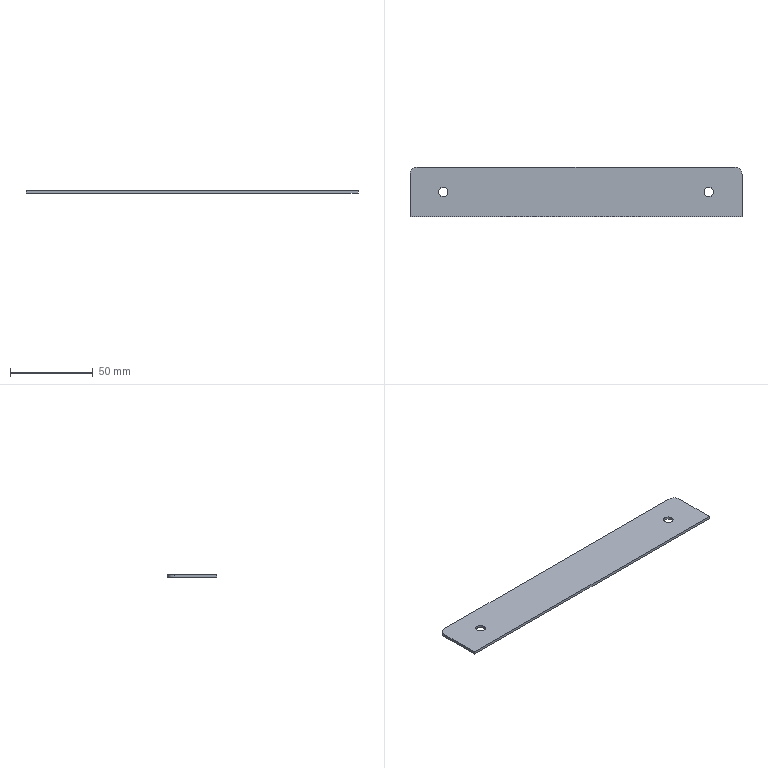Part | STEP file | [02]-11 | 1 solid | 12 faces | box 200 x 30 x 1.6 mm | volume 9501 mm3 | cylinder 6 | plane 6 | commonest cylinder face diameters 5.8 x4 9.2 x2
STEP:
#1=CARTESIAN_POINT('',(0.,0.,0.));
#2=DIRECTION('',(0.,0.,1.));
#3=DIRECTION('',(1.,0.,0.));
#4=AXIS2_PLACEMENT_3D('',#1,#2,#3);
#5=CARTESIAN_POINT('',(180.,17.9,1.6));
#6=VERTEX_POINT('',#5);
#7=CARTESIAN_POINT('',(180.,17.9,0.));
#8=VERTEX_POINT('',#7);
#9=CARTESIAN_POINT('',(180.,17.9,1.6));
#10=DIRECTION('',(0.,0.,-1.));
#11=VECTOR('',#10,1.);
#12=LINE('',#9,#11);
#13=CARTESIAN_POINT('',(180.,15.,1.6));
#14=DIRECTION('',(0.,0.,-1.));
#15=DIRECTION('',(0.,1.,0.));
#16=AXIS2_PLACEMENT_3D('',#13,#14,#15);
#17=CYLINDRICAL_SURFACE('',#16,2.9);
#18=CARTESIAN_POINT('',(6.283,0.));
#19=DIRECTION('',(0.,1.));
#20=VECTOR('',#19,1.);
#21=LINE('',#18,#20);
#22=(GEOMETRIC_REPRESENTATION_CONTEXT(2)PARAMETRIC_REPRESENTATION_CONTEXT()REPRESENTATION_CONTEXT('',''));
#23=DEFINITIONAL_REPRESENTATION('',(#21),#22);
#24=PCURVE('',#17,#23);
#25=CARTESIAN_POINT('',(180.,15.,1.6));
#26=DIRECTION('',(0.,0.,-1.));
#27=DIRECTION('',(0.,1.,0.));
#28=AXIS2_PLACEMENT_3D('',#25,#26,#27);
#29=CYLINDRICAL_SURFACE('',#28,2.9);
#30=CARTESIAN_POINT('',(0.,0.));
#31=DIRECTION('',(0.,1.));
#32=VECTOR('',#31,1.);
#33=LINE('',#30,#32);
#34=(GEOMETRIC_REPRESENTATION_CONTEXT(2)PARAMETRIC_REPRESENTATION_CONTEXT()REPRESENTATION_CONTEXT('',''));
#35=DEFINITIONAL_REPRESENTATION('',(#33),#34);
#36=PCURVE('',#29,#35);
#37=SURFACE_CURVE('',#12,(#24,#36),.PCURVE_S1.);
#38=EDGE_CURVE('',#6,#8,#37,.T.);
#39=ORIENTED_EDGE('',*,*,#38,.T.);
#40=CARTESIAN_POINT('',(180.,12.1,0.));
#41=VERTEX_POINT('',#40);
#42=CARTESIAN_POINT('',(180.,15.,0.));
#43=DIRECTION('',(0.,0.,1.));
#44=DIRECTION('',(0.,-1.,0.));
#45=AXIS2_PLACEMENT_3D('',#42,#43,#44);
#46=CIRCLE('',#45,2.9);
#47=CARTESIAN_POINT('',(9.425,1.6));
#48=DIRECTION('',(-1.,0.));
#49=VECTOR('',#48,1.);
#50=LINE('',#47,#49);
#51=(GEOMETRIC_REPRESENTATION_CONTEXT(2)PARAMETRIC_REPRESENTATION_CONTEXT()REPRESENTATION_CONTEXT('',''));
#52=DEFINITIONAL_REPRESENTATION('',(#50),#51);
#53=PCURVE('',#17,#52);
#54=CARTESIAN_POINT('',(100.,15.,0.));
#55=DIRECTION('',(0.,0.,-1.));
#56=DIRECTION('',(-1.,0.,0.));
#57=AXIS2_PLACEMENT_3D('',#54,#55,#56);
#58=PLANE('',#57);
#59=CARTESIAN_POINT('',(-80.,-2.9));
#60=CARTESIAN_POINT('',(-85.023,-2.9));
#61=CARTESIAN_POINT('',(-82.511,1.45));
#62=CARTESIAN_POINT('',(-80.,5.8));
#63=CARTESIAN_POINT('',(-77.489,1.45));
#64=CARTESIAN_POINT('',(-74.977,-2.9));
#65=CARTESIAN_POINT('',(-80.,-2.9));
#66=(BOUNDED_CURVE()B_SPLINE_CURVE(2,(#59,#60,#61,#62,#63,#64,#65),.UNSPECIFIED.,.T.,.F.)B_SPLINE_CURVE_WITH_KNOTS((1,2,2,2,2,1),(-2.094,0.,2.094,4.189,6.283,8.378),.UNSPECIFIED.)CURVE()GEOMETRIC_REPRESENTATION_ITEM()RATIONAL_B_SPLINE_CURVE((1.,0.5,1.,0.5,1.,0.5,1.))REPRESENTATION_ITEM(''));
#67=(GEOMETRIC_REPRESENTATION_CONTEXT(2)PARAMETRIC_REPRESENTATION_CONTEXT()REPRESENTATION_CONTEXT('',''));
#68=DEFINITIONAL_REPRESENTATION('',(#66),#67);
#69=PCURVE('',#58,#68);
#70=SURFACE_CURVE('',#46,(#53,#69),.PCURVE_S1.);
#71=EDGE_CURVE('',#8,#41,#70,.T.);
#72=ORIENTED_EDGE('',*,*,#71,.T.);
#73=CARTESIAN_POINT('',(180.,12.1,1.6));
#74=VERTEX_POINT('',#73);
#75=CARTESIAN_POINT('',(180.,12.1,1.6));
#76=DIRECTION('',(0.,0.,-1.));
#77=VECTOR('',#76,1.);
#78=LINE('',#75,#77);
#79=CARTESIAN_POINT('',(3.142,0.));
#80=DIRECTION('',(0.,1.));
#81=VECTOR('',#80,1.);
#82=LINE('',#79,#81);
#83=(GEOMETRIC_REPRESENTATION_CONTEXT(2)PARAMETRIC_REPRESENTATION_CONTEXT()REPRESENTATION_CONTEXT('',''));
#84=DEFINITIONAL_REPRESENTATION('',(#82),#83);
#85=PCURVE('',#17,#84);
#86=CARTESIAN_POINT('',(3.142,0.));
#87=DIRECTION('',(0.,1.));
#88=VECTOR('',#87,1.);
#89=LINE('',#86,#88);
#90=(GEOMETRIC_REPRESENTATION_CONTEXT(2)PARAMETRIC_REPRESENTATION_CONTEXT()REPRESENTATION_CONTEXT('',''));
#91=DEFINITIONAL_REPRESENTATION('',(#89),#90);
#92=PCURVE('',#29,#91);
#93=SURFACE_CURVE('',#78,(#85,#92),.PCURVE_S1.);
#94=EDGE_CURVE('',#74,#41,#93,.T.);
#95=ORIENTED_EDGE('',*,*,#94,.F.);
#96=CARTESIAN_POINT('',(180.,15.,1.6));
#97=DIRECTION('',(0.,0.,-1.));
#98=DIRECTION('',(0.,1.,0.));
#99=AXIS2_PLACEMENT_3D('',#96,#97,#98);
#100=CIRCLE('',#99,2.9);
#101=CARTESIAN_POINT('',(0.,0.));
#102=DIRECTION('',(1.,0.));
#103=VECTOR('',#102,1.);
#104=LINE('',#101,#103);
#105=(GEOMETRIC_REPRESENTATION_CONTEXT(2)PARAMETRIC_REPRESENTATION_CONTEXT()REPRESENTATION_CONTEXT('',''));
#106=DEFINITIONAL_REPRESENTATION('',(#104),#105);
#107=PCURVE('',#17,#106);
#108=CARTESIAN_POINT('',(100.,15.,1.6));
#109=DIRECTION('',(0.,0.,1.));
#110=DIRECTION('',(1.,0.,0.));
#111=AXIS2_PLACEMENT_3D('',#108,#109,#110);
#112=PLANE('',#111);
#113=CARTESIAN_POINT('',(80.,2.9));
#114=CARTESIAN_POINT('',(85.023,2.9));
#115=CARTESIAN_POINT('',(82.511,-1.45));
#116=CARTESIAN_POINT('',(80.,-5.8));
#117=CARTESIAN_POINT('',(77.489,-1.45));
#118=CARTESIAN_POINT('',(74.977,2.9));
#119=CARTESIAN_POINT('',(80.,2.9));
#120=(BOUNDED_CURVE()B_SPLINE_CURVE(2,(#113,#114,#115,#116,#117,#118,#119),.UNSPECIFIED.,.T.,.F.)B_SPLINE_CURVE_WITH_KNOTS((1,2,2,2,2,1),(-2.094,0.,2.094,4.189,6.283,8.378),.UNSPECIFIED.)CURVE()GEOMETRIC_REPRESENTATION_ITEM()RATIONAL_B_SPLINE_CURVE((1.,0.5,1.,0.5,1.,0.5,1.))REPRESENTATION_ITEM(''));
#121=(GEOMETRIC_REPRESENTATION_CONTEXT(2)PARAMETRIC_REPRESENTATION_CONTEXT()REPRESENTATION_CONTEXT('',''));
#122=DEFINITIONAL_REPRESENTATION('',(#120),#121);
#123=PCURVE('',#112,#122);
#124=SURFACE_CURVE('',#100,(#107,#123),.PCURVE_S1.);
#125=EDGE_CURVE('',#74,#6,#124,.T.);
#126=ORIENTED_EDGE('',*,*,#125,.T.);
#127=EDGE_LOOP('',(#39,#72,#95,#126));
#128=FACE_BOUND('',#127,.F.);
#129=ADVANCED_FACE('',(#128),#17,.F.);
#130=CARTESIAN_POINT('',(20.,17.9,1.6));
#131=VERTEX_POINT('',#130);
#132=CARTESIAN_POINT('',(20.,17.9,0.));
#133=VERTEX_POINT('',#132);
#134=CARTESIAN_POINT('',(20.,17.9,1.6));
#135=DIRECTION('',(0.,0.,-1.));
#136=VECTOR('',#135,1.);
#137=LINE('',#134,#136);
#138=CARTESIAN_POINT('',(20.,15.,1.6));
#139=DIRECTION('',(0.,0.,-1.));
#140=DIRECTION('',(0.,1.,0.));
#141=AXIS2_PLACEMENT_3D('',#138,#139,#140);
#142=CYLINDRICAL_SURFACE('',#141,2.9);
#143=CARTESIAN_POINT('',(6.283,0.));
#144=DIRECTION('',(0.,1.));
#145=VECTOR('',#144,1.);
#146=LINE('',#143,#145);
#147=(GEOMETRIC_REPRESENTATION_CONTEXT(2)PARAMETRIC_REPRESENTATION_CONTEXT()REPRESENTATION_CONTEXT('',''));
#148=DEFINITIONAL_REPRESENTATION('',(#146),#147);
#149=PCURVE('',#142,#148);
#150=CARTESIAN_POINT('',(20.,15.,1.6));
#151=DIRECTION('',(0.,0.,-1.));
#152=DIRECTION('',(0.,1.,0.));
#153=AXIS2_PLACEMENT_3D('',#150,#151,#152);
#154=CYLINDRICAL_SURFACE('',#153,2.9);
#155=CARTESIAN_POINT('',(0.,0.));
#156=DIRECTION('',(0.,1.));
#157=VECTOR('',#156,1.);
#158=LINE('',#155,#157);
#159=(GEOMETRIC_REPRESENTATION_CONTEXT(2)PARAMETRIC_REPRESENTATION_CONTEXT()REPRESENTATION_CONTEXT('',''));
#160=DEFINITIONAL_REPRESENTATION('',(#158),#159);
#161=PCURVE('',#154,#160);
#162=SURFACE_CURVE('',#137,(#149,#161),.PCURVE_S1.);
#163=EDGE_CURVE('',#131,#133,#162,.T.);
#164=ORIENTED_EDGE('',*,*,#163,.T.);
#165=CARTESIAN_POINT('',(20.,12.1,0.));
#166=VERTEX_POINT('',#165);
#167=CARTESIAN_POINT('',(20.,15.,0.));
#168=DIRECTION('',(0.,0.,1.));
#169=DIRECTION('',(0.,-1.,0.));
#170=AXIS2_PLACEMENT_3D('',#167,#168,#169);
#171=CIRCLE('',#170,2.9);
#172=CARTESIAN_POINT('',(9.425,1.6));
#173=DIRECTION('',(-1.,0.));
#174=VECTOR('',#173,1.);
#175=LINE('',#172,#174);
#176=(GEOMETRIC_REPRESENTATION_CONTEXT(2)PARAMETRIC_REPRESENTATION_CONTEXT()REPRESENTATION_CONTEXT('',''));
#177=DEFINITIONAL_REPRESENTATION('',(#175),#176);
#178=PCURVE('',#142,#177);
#179=CARTESIAN_POINT('',(80.,-2.9));
#180=CARTESIAN_POINT('',(74.977,-2.9));
#181=CARTESIAN_POINT('',(77.489,1.45));
#182=CARTESIAN_POINT('',(80.,5.8));
#183=CARTESIAN_POINT('',(82.511,1.45));
#184=CARTESIAN_POINT('',(85.023,-2.9));
#185=CARTESIAN_POINT('',(80.,-2.9));
#186=(BOUNDED_CURVE()B_SPLINE_CURVE(2,(#179,#180,#181,#182,#183,#184,#185),.UNSPECIFIED.,.T.,.F.)B_SPLINE_CURVE_WITH_KNOTS((1,2,2,2,2,1),(-2.094,0.,2.094,4.189,6.283,8.378),.UNSPECIFIED.)CURVE()GEOMETRIC_REPRESENTATION_ITEM()RATIONAL_B_SPLINE_CURVE((1.,0.5,1.,0.5,1.,0.5,1.))REPRESENTATION_ITEM(''));
#187=(GEOMETRIC_REPRESENTATION_CONTEXT(2)PARAMETRIC_REPRESENTATION_CONTEXT()REPRESENTATION_CONTEXT('',''));
#188=DEFINITIONAL_REPRESENTATION('',(#186),#187);
#189=PCURVE('',#58,#188);
#190=SURFACE_CURVE('',#171,(#178,#189),.PCURVE_S1.);
#191=EDGE_CURVE('',#133,#166,#190,.T.);
#192=ORIENTED_EDGE('',*,*,#191,.T.);
#193=CARTESIAN_POINT('',(20.,12.1,1.6));
#194=VERTEX_POINT('',#193);
#195=CARTESIAN_POINT('',(20.,12.1,1.6));
#196=DIRECTION('',(0.,0.,-1.));
#197=VECTOR('',#196,1.);
#198=LINE('',#195,#197);
#199=CARTESIAN_POINT('',(3.142,0.));
#200=DIRECTION('',(0.,1.));
#201=VECTOR('',#200,1.);
#202=LINE('',#199,#201);
#203=(GEOMETRIC_REPRESENTATION_CONTEXT(2)PARAMETRIC_REPRESENTATION_CONTEXT()REPRESENTATION_CONTEXT('',''));
#204=DEFINITIONAL_REPRESENTATION('',(#202),#203);
#205=PCURVE('',#142,#204);
#206=CARTESIAN_POINT('',(3.142,0.));
#207=DIRECTION('',(0.,1.));
#208=VECTOR('',#207,1.);
#209=LINE('',#206,#208);
#210=(GEOMETRIC_REPRESENTATION_CONTEXT(2)PARAMETRIC_REPRESENTATION_CONTEXT()REPRESENTATION_CONTEXT('',''));
#211=DEFINITIONAL_REPRESENTATION('',(#209),#210);
#212=PCURVE('',#154,#211);
#213=SURFACE_CURVE('',#198,(#205,#212),.PCURVE_S1.);
#214=EDGE_CURVE('',#194,#166,#213,.T.);
#215=ORIENTED_EDGE('',*,*,#214,.F.);
#216=CARTESIAN_POINT('',(20.,15.,1.6));
#217=DIRECTION('',(0.,0.,-1.));
#218=DIRECTION('',(0.,1.,0.));
#219=AXIS2_PLACEMENT_3D('',#216,#217,#218);
#220=CIRCLE('',#219,2.9);
#221=CARTESIAN_POINT('',(0.,0.));
#222=DIRECTION('',(1.,0.));
#223=VECTOR('',#222,1.);
#224=LINE('',#221,#223);
#225=(GEOMETRIC_REPRESENTATION_CONTEXT(2)PARAMETRIC_REPRESENTATION_CONTEXT()REPRESENTATION_CONTEXT('',''));
#226=DEFINITIONAL_REPRESENTATION('',(#224),#225);
#227=PCURVE('',#142,#226);
#228=CARTESIAN_POINT('',(-80.,2.9));
#229=CARTESIAN_POINT('',(-74.977,2.9));
#230=CARTESIAN_POINT('',(-77.489,-1.45));
#231=CARTESIAN_POINT('',(-80.,-5.8));
#232=CARTESIAN_POINT('',(-82.511,-1.45));
#233=CARTESIAN_POINT('',(-85.023,2.9));
#234=CARTESIAN_POINT('',(-80.,2.9));
#235=(BOUNDED_CURVE()B_SPLINE_CURVE(2,(#228,#229,#230,#231,#232,#233,#234),.UNSPECIFIED.,.T.,.F.)B_SPLINE_CURVE_WITH_KNOTS((1,2,2,2,2,1),(-2.094,0.,2.094,4.189,6.283,8.378),.UNSPECIFIED.)CURVE()GEOMETRIC_REPRESENTATION_ITEM()RATIONAL_B_SPLINE_CURVE((1.,0.5,1.,0.5,1.,0.5,1.))REPRESENTATION_ITEM(''));
#236=(GEOMETRIC_REPRESENTATION_CONTEXT(2)PARAMETRIC_REPRESENTATION_CONTEXT()REPRESENTATION_CONTEXT('',''));
#237=DEFINITIONAL_REPRESENTATION('',(#235),#236);
#238=PCURVE('',#112,#237);
#239=SURFACE_CURVE('',#220,(#227,#238),.PCURVE_S1.);
#240=EDGE_CURVE('',#194,#131,#239,.T.);
#241=ORIENTED_EDGE('',*,*,#240,.T.);
#242=EDGE_LOOP('',(#164,#192,#215,#241));
#243=FACE_BOUND('',#242,.F.);
#244=ADVANCED_FACE('',(#243),#142,.F.);
#245=CARTESIAN_POINT('',(180.,15.,1.6));
#246=DIRECTION('',(0.,0.,-1.));
#247=DIRECTION('',(0.,1.,0.));
#248=AXIS2_PLACEMENT_3D('',#245,#246,#247);
#249=CIRCLE('',#248,2.9);
#250=CARTESIAN_POINT('',(80.,2.9));
#251=CARTESIAN_POINT('',(85.023,2.9));
#252=CARTESIAN_POINT('',(82.511,-1.45));
#253=CARTESIAN_POINT('',(80.,-5.8));
#254=CARTESIAN_POINT('',(77.489,-1.45));
#255=CARTESIAN_POINT('',(74.977,2.9));
#256=CARTESIAN_POINT('',(80.,2.9));
#257=(BOUNDED_CURVE()B_SPLINE_CURVE(2,(#250,#251,#252,#253,#254,#255,#256),.UNSPECIFIED.,.T.,.F.)B_SPLINE_CURVE_WITH_KNOTS((1,2,2,2,2,1),(-2.094,0.,2.094,4.189,6.283,8.378),.UNSPECIFIED.)CURVE()GEOMETRIC_REPRESENTATION_ITEM()RATIONAL_B_SPLINE_CURVE((1.,0.5,1.,0.5,1.,0.5,1.))REPRESENTATION_ITEM(''));
#258=(GEOMETRIC_REPRESENTATION_CONTEXT(2)PARAMETRIC_REPRESENTATION_CONTEXT()REPRESENTATION_CONTEXT('',''));
#259=DEFINITIONAL_REPRESENTATION('',(#257),#258);
#260=PCURVE('',#112,#259);
#261=CARTESIAN_POINT('',(0.,0.));
#262=DIRECTION('',(1.,0.));
#263=VECTOR('',#262,1.);
#264=LINE('',#261,#263);
#265=(GEOMETRIC_REPRESENTATION_CONTEXT(2)PARAMETRIC_REPRESENTATION_CONTEXT()REPRESENTATION_CONTEXT('',''));
#266=DEFINITIONAL_REPRESENTATION('',(#264),#265);
#267=PCURVE('',#29,#266);
#268=SURFACE_CURVE('',#249,(#260,#267),.PCURVE_S1.);
#269=EDGE_CURVE('',#6,#74,#268,.T.);
#270=ORIENTED_EDGE('',*,*,#269,.T.);
#271=ORIENTED_EDGE('',*,*,#125,.T.);
#272=EDGE_LOOP('',(#270,#271));
#273=FACE_BOUND('',#272,.T.);
#274=CARTESIAN_POINT('',(20.,15.,1.6));
#275=DIRECTION('',(0.,0.,-1.));
#276=DIRECTION('',(0.,1.,0.));
#277=AXIS2_PLACEMENT_3D('',#274,#275,#276);
#278=CIRCLE('',#277,2.9);
#279=CARTESIAN_POINT('',(-80.,2.9));
#280=CARTESIAN_POINT('',(-74.977,2.9));
#281=CARTESIAN_POINT('',(-77.489,-1.45));
#282=CARTESIAN_POINT('',(-80.,-5.8));
#283=CARTESIAN_POINT('',(-82.511,-1.45));
#284=CARTESIAN_POINT('',(-85.023,2.9));
#285=CARTESIAN_POINT('',(-80.,2.9));
#286=(BOUNDED_CURVE()B_SPLINE_CURVE(2,(#279,#280,#281,#282,#283,#284,#285),.UNSPECIFIED.,.T.,.F.)B_SPLINE_CURVE_WITH_KNOTS((1,2,2,2,2,1),(-2.094,0.,2.094,4.189,6.283,8.378),.UNSPECIFIED.)CURVE()GEOMETRIC_REPRESENTATION_ITEM()RATIONAL_B_SPLINE_CURVE((1.,0.5,1.,0.5,1.,0.5,1.))REPRESENTATION_ITEM(''));
#287=(GEOMETRIC_REPRESENTATION_CONTEXT(2)PARAMETRIC_REPRESENTATION_CONTEXT()REPRESENTATION_CONTEXT('',''));
#288=DEFINITIONAL_REPRESENTATION('',(#286),#287);
#289=PCURVE('',#112,#288);
#290=CARTESIAN_POINT('',(0.,0.));
#291=DIRECTION('',(1.,0.));
#292=VECTOR('',#291,1.);
#293=LINE('',#290,#292);
#294=(GEOMETRIC_REPRESENTATION_CONTEXT(2)PARAMETRIC_REPRESENTATION_CONTEXT()REPRESENTATION_CONTEXT('',''));
#295=DEFINITIONAL_REPRESENTATION('',(#293),#294);
#296=PCURVE('',#154,#295);
#297=SURFACE_CURVE('',#278,(#289,#296),.PCURVE_S1.);
#298=EDGE_CURVE('',#131,#194,#297,.T.);
#299=ORIENTED_EDGE('',*,*,#298,.T.);
#300=ORIENTED_EDGE('',*,*,#240,.T.);
#301=EDGE_LOOP('',(#299,#300));
#302=FACE_BOUND('',#301,.T.);
#303=CARTESIAN_POINT('',(200.,25.4,1.6));
#304=VERTEX_POINT('',#303);
#305=CARTESIAN_POINT('',(200.,0.,1.6));
#306=VERTEX_POINT('',#305);
#307=CARTESIAN_POINT('',(200.,15.,1.6));
#308=DIRECTION('',(0.,-1.,0.));
#309=VECTOR('',#308,1.);
#310=LINE('',#307,#309);
#311=CARTESIAN_POINT('',(100.,0.));
#312=DIRECTION('',(0.,-1.));
#313=VECTOR('',#312,1.);
#314=LINE('',#311,#313);
#315=(GEOMETRIC_REPRESENTATION_CONTEXT(2)PARAMETRIC_REPRESENTATION_CONTEXT()REPRESENTATION_CONTEXT('',''));
#316=DEFINITIONAL_REPRESENTATION('',(#314),#315);
#317=PCURVE('',#112,#316);
#318=CARTESIAN_POINT('',(200.,15.,0.));
#319=DIRECTION('',(1.,0.,0.));
#320=DIRECTION('',(0.,0.,-1.));
#321=AXIS2_PLACEMENT_3D('',#318,#319,#320);
#322=PLANE('',#321);
#323=CARTESIAN_POINT('',(-1.6,0.));
#324=DIRECTION('',(0.,-1.));
#325=VECTOR('',#324,1.);
#326=LINE('',#323,#325);
#327=(GEOMETRIC_REPRESENTATION_CONTEXT(2)PARAMETRIC_REPRESENTATION_CONTEXT()REPRESENTATION_CONTEXT('',''));
#328=DEFINITIONAL_REPRESENTATION('',(#326),#327);
#329=PCURVE('',#322,#328);
#330=SURFACE_CURVE('',#310,(#317,#329),.PCURVE_S1.);
#331=EDGE_CURVE('',#304,#306,#330,.T.);
#332=ORIENTED_EDGE('',*,*,#331,.F.);
#333=CARTESIAN_POINT('',(195.4,30.,1.6));
#334=VERTEX_POINT('',#333);
#335=CARTESIAN_POINT('',(195.4,25.4,1.6));
#336=DIRECTION('',(0.,0.,1.));
#337=DIRECTION('',(1.,0.,0.));
#338=AXIS2_PLACEMENT_3D('',#335,#336,#337);
#339=CIRCLE('',#338,4.6);
#340=CARTESIAN_POINT('',(95.4,10.4));
#341=DIRECTION('',(1.,0.));
#342=AXIS2_PLACEMENT_2D('',#340,#341);
#343=CIRCLE('',#342,4.6);
#344=(GEOMETRIC_REPRESENTATION_CONTEXT(2)PARAMETRIC_REPRESENTATION_CONTEXT()REPRESENTATION_CONTEXT('',''));
#345=DEFINITIONAL_REPRESENTATION('',(#343),#344);
#346=PCURVE('',#112,#345);
#347=CARTESIAN_POINT('',(195.4,25.4,0.));
#348=DIRECTION('',(0.,0.,1.));
#349=DIRECTION('',(1.,0.,0.));
#350=AXIS2_PLACEMENT_3D('',#347,#348,#349);
#351=CYLINDRICAL_SURFACE('',#350,4.6);
#352=CARTESIAN_POINT('',(0.,1.6));
#353=DIRECTION('',(1.,0.));
#354=VECTOR('',#353,1.);
#355=LINE('',#352,#354);
#356=(GEOMETRIC_REPRESENTATION_CONTEXT(2)PARAMETRIC_REPRESENTATION_CONTEXT()REPRESENTATION_CONTEXT('',''));
#357=DEFINITIONAL_REPRESENTATION('',(#355),#356);
#358=PCURVE('',#351,#357);
#359=SURFACE_CURVE('',#339,(#346,#358),.PCURVE_S1.);
#360=EDGE_CURVE('',#304,#334,#359,.T.);
#361=ORIENTED_EDGE('',*,*,#360,.T.);
#362=CARTESIAN_POINT('',(4.6,30.,1.6));
#363=VERTEX_POINT('',#362);
#364=CARTESIAN_POINT('',(100.,30.,1.6));
#365=DIRECTION('',(1.,0.,0.));
#366=VECTOR('',#365,1.);
#367=LINE('',#364,#366);
#368=CARTESIAN_POINT('',(0.,15.));
#369=DIRECTION('',(1.,0.));
#370=VECTOR('',#369,1.);
#371=LINE('',#368,#370);
#372=(GEOMETRIC_REPRESENTATION_CONTEXT(2)PARAMETRIC_REPRESENTATION_CONTEXT()REPRESENTATION_CONTEXT('',''));
#373=DEFINITIONAL_REPRESENTATION('',(#371),#372);
#374=PCURVE('',#112,#373);
#375=CARTESIAN_POINT('',(100.,30.,0.));
#376=DIRECTION('',(0.,1.,0.));
#377=DIRECTION('',(0.,0.,1.));
#378=AXIS2_PLACEMENT_3D('',#375,#376,#377);
#379=PLANE('',#378);
#380=CARTESIAN_POINT('',(1.6,0.));
#381=DIRECTION('',(0.,1.));
#382=VECTOR('',#381,1.);
#383=LINE('',#380,#382);
#384=(GEOMETRIC_REPRESENTATION_CONTEXT(2)PARAMETRIC_REPRESENTATION_CONTEXT()REPRESENTATION_CONTEXT('',''));
#385=DEFINITIONAL_REPRESENTATION('',(#383),#384);
#386=PCURVE('',#379,#385);
#387=SURFACE_CURVE('',#367,(#374,#386),.PCURVE_S1.);
#388=EDGE_CURVE('',#363,#334,#387,.T.);
#389=ORIENTED_EDGE('',*,*,#388,.F.);
#390=CARTESIAN_POINT('',(0.,25.4,1.6));
#391=VERTEX_POINT('',#390);
#392=CARTESIAN_POINT('',(4.6,25.4,1.6));
#393=DIRECTION('',(0.,0.,1.));
#394=DIRECTION('',(1.,0.,0.));
#395=AXIS2_PLACEMENT_3D('',#392,#393,#394);
#396=CIRCLE('',#395,4.6);
#397=CARTESIAN_POINT('',(-95.4,10.4));
#398=DIRECTION('',(1.,0.));
#399=AXIS2_PLACEMENT_2D('',#397,#398);
#400=CIRCLE('',#399,4.6);
#401=(GEOMETRIC_REPRESENTATION_CONTEXT(2)PARAMETRIC_REPRESENTATION_CONTEXT()REPRESENTATION_CONTEXT('',''));
#402=DEFINITIONAL_REPRESENTATION('',(#400),#401);
#403=PCURVE('',#112,#402);
#404=CARTESIAN_POINT('',(4.6,25.4,0.));
#405=DIRECTION('',(0.,0.,1.));
#406=DIRECTION('',(1.,0.,0.));
#407=AXIS2_PLACEMENT_3D('',#404,#405,#406);
#408=CYLINDRICAL_SURFACE('',#407,4.6);
#409=CARTESIAN_POINT('',(0.,1.6));
#410=DIRECTION('',(1.,0.));
#411=VECTOR('',#410,1.);
#412=LINE('',#409,#411);
#413=(GEOMETRIC_REPRESENTATION_CONTEXT(2)PARAMETRIC_REPRESENTATION_CONTEXT()REPRESENTATION_CONTEXT('',''));
#414=DEFINITIONAL_REPRESENTATION('',(#412),#413);
#415=PCURVE('',#408,#414);
#416=SURFACE_CURVE('',#396,(#403,#415),.PCURVE_S1.);
#417=EDGE_CURVE('',#363,#391,#416,.T.);
#418=ORIENTED_EDGE('',*,*,#417,.T.);
#419=CARTESIAN_POINT('',(0.,0.,1.6));
#420=VERTEX_POINT('',#419);
#421=CARTESIAN_POINT('',(0.,15.,1.6));
#422=DIRECTION('',(0.,1.,0.));
#423=VECTOR('',#422,1.);
#424=LINE('',#421,#423);
#425=CARTESIAN_POINT('',(-100.,0.));
#426=DIRECTION('',(0.,1.));
#427=VECTOR('',#426,1.);
#428=LINE('',#425,#427);
#429=(GEOMETRIC_REPRESENTATION_CONTEXT(2)PARAMETRIC_REPRESENTATION_CONTEXT()REPRESENTATION_CONTEXT('',''));
#430=DEFINITIONAL_REPRESENTATION('',(#428),#429);
#431=PCURVE('',#112,#430);
#432=CARTESIAN_POINT('',(0.,15.,0.));
#433=DIRECTION('',(-1.,0.,0.));
#434=DIRECTION('',(0.,0.,1.));
#435=AXIS2_PLACEMENT_3D('',#432,#433,#434);
#436=PLANE('',#435);
#437=CARTESIAN_POINT('',(1.6,0.));
#438=DIRECTION('',(0.,1.));
#439=VECTOR('',#438,1.);
#440=LINE('',#437,#439);
#441=(GEOMETRIC_REPRESENTATION_CONTEXT(2)PARAMETRIC_REPRESENTATION_CONTEXT()REPRESENTATION_CONTEXT('',''));
#442=DEFINITIONAL_REPRESENTATION('',(#440),#441);
#443=PCURVE('',#436,#442);
#444=SURFACE_CURVE('',#424,(#431,#443),.PCURVE_S1.);
#445=EDGE_CURVE('',#420,#391,#444,.T.);
#446=ORIENTED_EDGE('',*,*,#445,.F.);
#447=CARTESIAN_POINT('',(100.,0.,1.6));
#448=DIRECTION('',(-1.,0.,0.));
#449=VECTOR('',#448,1.);
#450=LINE('',#447,#449);
#451=CARTESIAN_POINT('',(0.,-15.));
#452=DIRECTION('',(-1.,0.));
#453=VECTOR('',#452,1.);
#454=LINE('',#451,#453);
#455=(GEOMETRIC_REPRESENTATION_CONTEXT(2)PARAMETRIC_REPRESENTATION_CONTEXT()REPRESENTATION_CONTEXT('',''));
#456=DEFINITIONAL_REPRESENTATION('',(#454),#455);
#457=PCURVE('',#112,#456);
#458=CARTESIAN_POINT('',(100.,0.,0.));
#459=DIRECTION('',(0.,-1.,0.));
#460=DIRECTION('',(0.,0.,-1.));
#461=AXIS2_PLACEMENT_3D('',#458,#459,#460);
#462=PLANE('',#461);
#463=CARTESIAN_POINT('',(-1.6,0.));
#464=DIRECTION('',(0.,-1.));
#465=VECTOR('',#464,1.);
#466=LINE('',#463,#465);
#467=(GEOMETRIC_REPRESENTATION_CONTEXT(2)PARAMETRIC_REPRESENTATION_CONTEXT()REPRESENTATION_CONTEXT('',''));
#468=DEFINITIONAL_REPRESENTATION('',(#466),#467);
#469=PCURVE('',#462,#468);
#470=SURFACE_CURVE('',#450,(#457,#469),.PCURVE_S1.);
#471=EDGE_CURVE('',#306,#420,#470,.T.);
#472=ORIENTED_EDGE('',*,*,#471,.F.);
#473=EDGE_LOOP('',(#332,#361,#389,#418,#446,#472));
#474=FACE_BOUND('',#473,.T.);
#475=ADVANCED_FACE('',(#273,#302,#474),#112,.T.);
#476=CARTESIAN_POINT('',(200.,0.,0.));
#477=VERTEX_POINT('',#476);
#478=CARTESIAN_POINT('',(200.,0.,0.));
#479=DIRECTION('',(0.,0.,1.));
#480=VECTOR('',#479,1.);
#481=LINE('',#478,#480);
#482=CARTESIAN_POINT('',(0.,100.));
#483=DIRECTION('',(-1.,0.));
#484=VECTOR('',#483,1.);
#485=LINE('',#482,#484);
#486=(GEOMETRIC_REPRESENTATION_CONTEXT(2)PARAMETRIC_REPRESENTATION_CONTEXT()REPRESENTATION_CONTEXT('',''));
#487=DEFINITIONAL_REPRESENTATION('',(#485),#486);
#488=PCURVE('',#462,#487);
#489=CARTESIAN_POINT('',(0.,-15.));
#490=DIRECTION('',(-1.,0.));
#491=VECTOR('',#490,1.);
#492=LINE('',#489,#491);
#493=(GEOMETRIC_REPRESENTATION_CONTEXT(2)PARAMETRIC_REPRESENTATION_CONTEXT()REPRESENTATION_CONTEXT('',''));
#494=DEFINITIONAL_REPRESENTATION('',(#492),#493);
#495=PCURVE('',#322,#494);
#496=SURFACE_CURVE('',#481,(#488,#495),.PCURVE_S1.);
#497=EDGE_CURVE('',#477,#306,#496,.T.);
#498=ORIENTED_EDGE('',*,*,#497,.T.);
#499=ORIENTED_EDGE('',*,*,#471,.T.);
#500=CARTESIAN_POINT('',(0.,0.,0.));
#501=VERTEX_POINT('',#500);
#502=CARTESIAN_POINT('',(0.,0.,0.));
#503=DIRECTION('',(0.,0.,1.));
#504=VECTOR('',#503,1.);
#505=LINE('',#502,#504);
#506=CARTESIAN_POINT('',(0.,-100.));
#507=DIRECTION('',(-1.,0.));
#508=VECTOR('',#507,1.);
#509=LINE('',#506,#508);
#510=(GEOMETRIC_REPRESENTATION_CONTEXT(2)PARAMETRIC_REPRESENTATION_CONTEXT()REPRESENTATION_CONTEXT('',''));
#511=DEFINITIONAL_REPRESENTATION('',(#509),#510);
#512=PCURVE('',#462,#511);
#513=CARTESIAN_POINT('',(0.,-15.));
#514=DIRECTION('',(1.,0.));
#515=VECTOR('',#514,1.);
#516=LINE('',#513,#515);
#517=(GEOMETRIC_REPRESENTATION_CONTEXT(2)PARAMETRIC_REPRESENTATION_CONTEXT()REPRESENTATION_CONTEXT('',''));
#518=DEFINITIONAL_REPRESENTATION('',(#516),#517);
#519=PCURVE('',#436,#518);
#520=SURFACE_CURVE('',#505,(#512,#519),.PCURVE_S1.);
#521=EDGE_CURVE('',#501,#420,#520,.T.);
#522=ORIENTED_EDGE('',*,*,#521,.F.);
#523=CARTESIAN_POINT('',(100.,0.,0.));
#524=DIRECTION('',(1.,0.,0.));
#525=VECTOR('',#524,1.);
#526=LINE('',#523,#525);
#527=CARTESIAN_POINT('',(0.,0.));
#528=DIRECTION('',(0.,1.));
#529=VECTOR('',#528,1.);
#530=LINE('',#527,#529);
#531=(GEOMETRIC_REPRESENTATION_CONTEXT(2)PARAMETRIC_REPRESENTATION_CONTEXT()REPRESENTATION_CONTEXT('',''));
#532=DEFINITIONAL_REPRESENTATION('',(#530),#531);
#533=PCURVE('',#462,#532);
#534=CARTESIAN_POINT('',(0.,-15.));
#535=DIRECTION('',(-1.,0.));
#536=VECTOR('',#535,1.);
#537=LINE('',#534,#536);
#538=(GEOMETRIC_REPRESENTATION_CONTEXT(2)PARAMETRIC_REPRESENTATION_CONTEXT()REPRESENTATION_CONTEXT('',''));
#539=DEFINITIONAL_REPRESENTATION('',(#537),#538);
#540=PCURVE('',#58,#539);
#541=SURFACE_CURVE('',#526,(#533,#540),.PCURVE_S1.);
#542=EDGE_CURVE('',#501,#477,#541,.T.);
#543=ORIENTED_EDGE('',*,*,#542,.T.);
#544=EDGE_LOOP('',(#498,#499,#522,#543));
#545=FACE_BOUND('',#544,.T.);
#546=ADVANCED_FACE('',(#545),#462,.T.);
#547=ORIENTED_EDGE('',*,*,#445,.T.);
#548=CARTESIAN_POINT('',(0.,25.4,0.));
#549=VERTEX_POINT('',#548);
#550=CARTESIAN_POINT('',(0.,25.4,0.));
#551=DIRECTION('',(0.,0.,-1.));
#552=VECTOR('',#551,1.);
#553=LINE('',#550,#552);
#554=CARTESIAN_POINT('',(0.,10.4));
#555=DIRECTION('',(-1.,0.));
#556=VECTOR('',#555,1.);
#557=LINE('',#554,#556);
#558=(GEOMETRIC_REPRESENTATION_CONTEXT(2)PARAMETRIC_REPRESENTATION_CONTEXT()REPRESENTATION_CONTEXT('',''));
#559=DEFINITIONAL_REPRESENTATION('',(#557),#558);
#560=PCURVE('',#436,#559);
#561=CARTESIAN_POINT('',(3.142,0.));
#562=DIRECTION('',(0.,-1.));
#563=VECTOR('',#562,1.);
#564=LINE('',#561,#563);
#565=(GEOMETRIC_REPRESENTATION_CONTEXT(2)PARAMETRIC_REPRESENTATION_CONTEXT()REPRESENTATION_CONTEXT('',''));
#566=DEFINITIONAL_REPRESENTATION('',(#564),#565);
#567=PCURVE('',#408,#566);
#568=SURFACE_CURVE('',#553,(#560,#567),.PCURVE_S1.);
#569=EDGE_CURVE('',#391,#549,#568,.T.);
#570=ORIENTED_EDGE('',*,*,#569,.T.);
#571=CARTESIAN_POINT('',(0.,15.,0.));
#572=DIRECTION('',(0.,-1.,0.));
#573=VECTOR('',#572,1.);
#574=LINE('',#571,#573);
#575=CARTESIAN_POINT('',(0.,0.));
#576=DIRECTION('',(0.,-1.));
#577=VECTOR('',#576,1.);
#578=LINE('',#575,#577);
#579=(GEOMETRIC_REPRESENTATION_CONTEXT(2)PARAMETRIC_REPRESENTATION_CONTEXT()REPRESENTATION_CONTEXT('',''));
#580=DEFINITIONAL_REPRESENTATION('',(#578),#579);
#581=PCURVE('',#436,#580);
#582=CARTESIAN_POINT('',(100.,0.));
#583=DIRECTION('',(0.,-1.));
#584=VECTOR('',#583,1.);
#585=LINE('',#582,#584);
#586=(GEOMETRIC_REPRESENTATION_CONTEXT(2)PARAMETRIC_REPRESENTATION_CONTEXT()REPRESENTATION_CONTEXT('',''));
#587=DEFINITIONAL_REPRESENTATION('',(#585),#586);
#588=PCURVE('',#58,#587);
#589=SURFACE_CURVE('',#574,(#581,#588),.PCURVE_S1.);
#590=EDGE_CURVE('',#549,#501,#589,.T.);
#591=ORIENTED_EDGE('',*,*,#590,.T.);
#592=ORIENTED_EDGE('',*,*,#521,.T.);
#593=EDGE_LOOP('',(#547,#570,#591,#592));
#594=FACE_BOUND('',#593,.T.);
#595=ADVANCED_FACE('',(#594),#436,.T.);
#596=ORIENTED_EDGE('',*,*,#388,.T.);
#597=CARTESIAN_POINT('',(195.4,30.,0.));
#598=VERTEX_POINT('',#597);
#599=CARTESIAN_POINT('',(195.4,30.,0.));
#600=DIRECTION('',(0.,0.,-1.));
#601=VECTOR('',#600,1.);
#602=LINE('',#599,#601);
#603=CARTESIAN_POINT('',(0.,95.4));
#604=DIRECTION('',(-1.,0.));
#605=VECTOR('',#604,1.);
#606=LINE('',#603,#605);
#607=(GEOMETRIC_REPRESENTATION_CONTEXT(2)PARAMETRIC_REPRESENTATION_CONTEXT()REPRESENTATION_CONTEXT('',''));
#608=DEFINITIONAL_REPRESENTATION('',(#606),#607);
#609=PCURVE('',#379,#608);
#610=CARTESIAN_POINT('',(1.571,0.));
#611=DIRECTION('',(0.,-1.));
#612=VECTOR('',#611,1.);
#613=LINE('',#610,#612);
#614=(GEOMETRIC_REPRESENTATION_CONTEXT(2)PARAMETRIC_REPRESENTATION_CONTEXT()REPRESENTATION_CONTEXT('',''));
#615=DEFINITIONAL_REPRESENTATION('',(#613),#614);
#616=PCURVE('',#351,#615);
#617=SURFACE_CURVE('',#602,(#609,#616),.PCURVE_S1.);
#618=EDGE_CURVE('',#334,#598,#617,.T.);
#619=ORIENTED_EDGE('',*,*,#618,.T.);
#620=CARTESIAN_POINT('',(4.6,30.,0.));
#621=VERTEX_POINT('',#620);
#622=CARTESIAN_POINT('',(100.,30.,0.));
#623=DIRECTION('',(-1.,0.,0.));
#624=VECTOR('',#623,1.);
#625=LINE('',#622,#624);
#626=CARTESIAN_POINT('',(0.,0.));
#627=DIRECTION('',(0.,-1.));
#628=VECTOR('',#627,1.);
#629=LINE('',#626,#628);
#630=(GEOMETRIC_REPRESENTATION_CONTEXT(2)PARAMETRIC_REPRESENTATION_CONTEXT()REPRESENTATION_CONTEXT('',''));
#631=DEFINITIONAL_REPRESENTATION('',(#629),#630);
#632=PCURVE('',#379,#631);
#633=CARTESIAN_POINT('',(0.,15.));
#634=DIRECTION('',(1.,0.));
#635=VECTOR('',#634,1.);
#636=LINE('',#633,#635);
#637=(GEOMETRIC_REPRESENTATION_CONTEXT(2)PARAMETRIC_REPRESENTATION_CONTEXT()REPRESENTATION_CONTEXT('',''));
#638=DEFINITIONAL_REPRESENTATION('',(#636),#637);
#639=PCURVE('',#58,#638);
#640=SURFACE_CURVE('',#625,(#632,#639),.PCURVE_S1.);
#641=EDGE_CURVE('',#598,#621,#640,.T.);
#642=ORIENTED_EDGE('',*,*,#641,.T.);
#643=CARTESIAN_POINT('',(4.6,30.,0.));
#644=DIRECTION('',(0.,0.,1.));
#645=VECTOR('',#644,1.);
#646=LINE('',#643,#645);
#647=CARTESIAN_POINT('',(0.,-95.4));
#648=DIRECTION('',(1.,0.));
#649=VECTOR('',#648,1.);
#650=LINE('',#647,#649);
#651=(GEOMETRIC_REPRESENTATION_CONTEXT(2)PARAMETRIC_REPRESENTATION_CONTEXT()REPRESENTATION_CONTEXT('',''));
#652=DEFINITIONAL_REPRESENTATION('',(#650),#651);
#653=PCURVE('',#379,#652);
#654=CARTESIAN_POINT('',(1.571,0.));
#655=DIRECTION('',(0.,1.));
#656=VECTOR('',#655,1.);
#657=LINE('',#654,#656);
#658=(GEOMETRIC_REPRESENTATION_CONTEXT(2)PARAMETRIC_REPRESENTATION_CONTEXT()REPRESENTATION_CONTEXT('',''));
#659=DEFINITIONAL_REPRESENTATION('',(#657),#658);
#660=PCURVE('',#408,#659);
#661=SURFACE_CURVE('',#646,(#653,#660),.PCURVE_S1.);
#662=EDGE_CURVE('',#621,#363,#661,.T.);
#663=ORIENTED_EDGE('',*,*,#662,.T.);
#664=EDGE_LOOP('',(#596,#619,#642,#663));
#665=FACE_BOUND('',#664,.T.);
#666=ADVANCED_FACE('',(#665),#379,.T.);
#667=ORIENTED_EDGE('',*,*,#71,.T.);
#668=CARTESIAN_POINT('',(180.,15.,0.));
#669=DIRECTION('',(0.,0.,1.));
#670=DIRECTION('',(0.,-1.,0.));
#671=AXIS2_PLACEMENT_3D('',#668,#669,#670);
#672=CIRCLE('',#671,2.9);
#673=CARTESIAN_POINT('',(-80.,-2.9));
#674=CARTESIAN_POINT('',(-85.023,-2.9));
#675=CARTESIAN_POINT('',(-82.511,1.45));
#676=CARTESIAN_POINT('',(-80.,5.8));
#677=CARTESIAN_POINT('',(-77.489,1.45));
#678=CARTESIAN_POINT('',(-74.977,-2.9));
#679=CARTESIAN_POINT('',(-80.,-2.9));
#680=(BOUNDED_CURVE()B_SPLINE_CURVE(2,(#673,#674,#675,#676,#677,#678,#679),.UNSPECIFIED.,.T.,.F.)B_SPLINE_CURVE_WITH_KNOTS((1,2,2,2,2,1),(-2.094,0.,2.094,4.189,6.283,8.378),.UNSPECIFIED.)CURVE()GEOMETRIC_REPRESENTATION_ITEM()RATIONAL_B_SPLINE_CURVE((1.,0.5,1.,0.5,1.,0.5,1.))REPRESENTATION_ITEM(''));
#681=(GEOMETRIC_REPRESENTATION_CONTEXT(2)PARAMETRIC_REPRESENTATION_CONTEXT()REPRESENTATION_CONTEXT('',''));
#682=DEFINITIONAL_REPRESENTATION('',(#680),#681);
#683=PCURVE('',#58,#682);
#684=CARTESIAN_POINT('',(3.142,1.6));
#685=DIRECTION('',(-1.,0.));
#686=VECTOR('',#685,1.);
#687=LINE('',#684,#686);
#688=(GEOMETRIC_REPRESENTATION_CONTEXT(2)PARAMETRIC_REPRESENTATION_CONTEXT()REPRESENTATION_CONTEXT('',''));
#689=DEFINITIONAL_REPRESENTATION('',(#687),#688);
#690=PCURVE('',#29,#689);
#691=SURFACE_CURVE('',#672,(#683,#690),.PCURVE_S1.);
#692=EDGE_CURVE('',#41,#8,#691,.T.);
#693=ORIENTED_EDGE('',*,*,#692,.T.);
#694=EDGE_LOOP('',(#667,#693));
#695=FACE_BOUND('',#694,.T.);
#696=ORIENTED_EDGE('',*,*,#191,.T.);
#697=CARTESIAN_POINT('',(20.,15.,0.));
#698=DIRECTION('',(0.,0.,1.));
#699=DIRECTION('',(0.,-1.,0.));
#700=AXIS2_PLACEMENT_3D('',#697,#698,#699);
#701=CIRCLE('',#700,2.9);
#702=CARTESIAN_POINT('',(80.,-2.9));
#703=CARTESIAN_POINT('',(74.977,-2.9));
#704=CARTESIAN_POINT('',(77.489,1.45));
#705=CARTESIAN_POINT('',(80.,5.8));
#706=CARTESIAN_POINT('',(82.511,1.45));
#707=CARTESIAN_POINT('',(85.023,-2.9));
#708=CARTESIAN_POINT('',(80.,-2.9));
#709=(BOUNDED_CURVE()B_SPLINE_CURVE(2,(#702,#703,#704,#705,#706,#707,#708),.UNSPECIFIED.,.T.,.F.)B_SPLINE_CURVE_WITH_KNOTS((1,2,2,2,2,1),(-2.094,0.,2.094,4.189,6.283,8.378),.UNSPECIFIED.)CURVE()GEOMETRIC_REPRESENTATION_ITEM()RATIONAL_B_SPLINE_CURVE((1.,0.5,1.,0.5,1.,0.5,1.))REPRESENTATION_ITEM(''));
#710=(GEOMETRIC_REPRESENTATION_CONTEXT(2)PARAMETRIC_REPRESENTATION_CONTEXT()REPRESENTATION_CONTEXT('',''));
#711=DEFINITIONAL_REPRESENTATION('',(#709),#710);
#712=PCURVE('',#58,#711);
#713=CARTESIAN_POINT('',(3.142,1.6));
#714=DIRECTION('',(-1.,0.));
#715=VECTOR('',#714,1.);
#716=LINE('',#713,#715);
#717=(GEOMETRIC_REPRESENTATION_CONTEXT(2)PARAMETRIC_REPRESENTATION_CONTEXT()REPRESENTATION_CONTEXT('',''));
#718=DEFINITIONAL_REPRESENTATION('',(#716),#717);
#719=PCURVE('',#154,#718);
#720=SURFACE_CURVE('',#701,(#712,#719),.PCURVE_S1.);
#721=EDGE_CURVE('',#166,#133,#720,.T.);
#722=ORIENTED_EDGE('',*,*,#721,.T.);
#723=EDGE_LOOP('',(#696,#722));
#724=FACE_BOUND('',#723,.T.);
#725=ORIENTED_EDGE('',*,*,#641,.F.);
#726=CARTESIAN_POINT('',(200.,25.4,0.));
#727=VERTEX_POINT('',#726);
#728=CARTESIAN_POINT('',(195.4,25.4,0.));
#729=DIRECTION('',(0.,0.,-1.));
#730=DIRECTION('',(-1.,0.,0.));
#731=AXIS2_PLACEMENT_3D('',#728,#729,#730);
#732=CIRCLE('',#731,4.6);
#733=CARTESIAN_POINT('',(-95.4,10.4));
#734=DIRECTION('',(1.,0.));
#735=AXIS2_PLACEMENT_2D('',#733,#734);
#736=CIRCLE('',#735,4.6);
#737=(GEOMETRIC_REPRESENTATION_CONTEXT(2)PARAMETRIC_REPRESENTATION_CONTEXT()REPRESENTATION_CONTEXT('',''));
#738=DEFINITIONAL_REPRESENTATION('',(#736),#737);
#739=PCURVE('',#58,#738);
#740=CARTESIAN_POINT('',(3.142,0.));
#741=DIRECTION('',(-1.,0.));
#742=VECTOR('',#741,1.);
#743=LINE('',#740,#742);
#744=(GEOMETRIC_REPRESENTATION_CONTEXT(2)PARAMETRIC_REPRESENTATION_CONTEXT()REPRESENTATION_CONTEXT('',''));
#745=DEFINITIONAL_REPRESENTATION('',(#743),#744);
#746=PCURVE('',#351,#745);
#747=SURFACE_CURVE('',#732,(#739,#746),.PCURVE_S1.);
#748=EDGE_CURVE('',#598,#727,#747,.T.);
#749=ORIENTED_EDGE('',*,*,#748,.T.);
#750=CARTESIAN_POINT('',(200.,15.,0.));
#751=DIRECTION('',(0.,1.,0.));
#752=VECTOR('',#751,1.);
#753=LINE('',#750,#752);
#754=CARTESIAN_POINT('',(-100.,0.));
#755=DIRECTION('',(0.,1.));
#756=VECTOR('',#755,1.);
#757=LINE('',#754,#756);
#758=(GEOMETRIC_REPRESENTATION_CONTEXT(2)PARAMETRIC_REPRESENTATION_CONTEXT()REPRESENTATION_CONTEXT('',''));
#759=DEFINITIONAL_REPRESENTATION('',(#757),#758);
#760=PCURVE('',#58,#759);
#761=CARTESIAN_POINT('',(0.,0.));
#762=DIRECTION('',(0.,1.));
#763=VECTOR('',#762,1.);
#764=LINE('',#761,#763);
#765=(GEOMETRIC_REPRESENTATION_CONTEXT(2)PARAMETRIC_REPRESENTATION_CONTEXT()REPRESENTATION_CONTEXT('',''));
#766=DEFINITIONAL_REPRESENTATION('',(#764),#765);
#767=PCURVE('',#322,#766);
#768=SURFACE_CURVE('',#753,(#760,#767),.PCURVE_S1.);
#769=EDGE_CURVE('',#477,#727,#768,.T.);
#770=ORIENTED_EDGE('',*,*,#769,.F.);
#771=ORIENTED_EDGE('',*,*,#542,.F.);
#772=ORIENTED_EDGE('',*,*,#590,.F.);
#773=CARTESIAN_POINT('',(4.6,25.4,0.));
#774=DIRECTION('',(0.,0.,-1.));
#775=DIRECTION('',(-1.,0.,0.));
#776=AXIS2_PLACEMENT_3D('',#773,#774,#775);
#777=CIRCLE('',#776,4.6);
#778=CARTESIAN_POINT('',(95.4,10.4));
#779=DIRECTION('',(1.,0.));
#780=AXIS2_PLACEMENT_2D('',#778,#779);
#781=CIRCLE('',#780,4.6);
#782=(GEOMETRIC_REPRESENTATION_CONTEXT(2)PARAMETRIC_REPRESENTATION_CONTEXT()REPRESENTATION_CONTEXT('',''));
#783=DEFINITIONAL_REPRESENTATION('',(#781),#782);
#784=PCURVE('',#58,#783);
#785=CARTESIAN_POINT('',(3.142,0.));
#786=DIRECTION('',(-1.,0.));
#787=VECTOR('',#786,1.);
#788=LINE('',#785,#787);
#789=(GEOMETRIC_REPRESENTATION_CONTEXT(2)PARAMETRIC_REPRESENTATION_CONTEXT()REPRESENTATION_CONTEXT('',''));
#790=DEFINITIONAL_REPRESENTATION('',(#788),#789);
#791=PCURVE('',#408,#790);
#792=SURFACE_CURVE('',#777,(#784,#791),.PCURVE_S1.);
#793=EDGE_CURVE('',#549,#621,#792,.T.);
#794=ORIENTED_EDGE('',*,*,#793,.T.);
#795=EDGE_LOOP('',(#725,#749,#770,#771,#772,#794));
#796=FACE_BOUND('',#795,.T.);
#797=ADVANCED_FACE('',(#695,#724,#796),#58,.T.);
#798=ORIENTED_EDGE('',*,*,#769,.T.);
#799=CARTESIAN_POINT('',(200.,25.4,0.));
#800=DIRECTION('',(0.,0.,1.));
#801=VECTOR('',#800,1.);
#802=LINE('',#799,#801);
#803=CARTESIAN_POINT('',(0.,10.4));
#804=DIRECTION('',(-1.,0.));
#805=VECTOR('',#804,1.);
#806=LINE('',#803,#805);
#807=(GEOMETRIC_REPRESENTATION_CONTEXT(2)PARAMETRIC_REPRESENTATION_CONTEXT()REPRESENTATION_CONTEXT('',''));
#808=DEFINITIONAL_REPRESENTATION('',(#806),#807);
#809=PCURVE('',#322,#808);
#810=CARTESIAN_POINT('',(0.,0.));
#811=DIRECTION('',(0.,1.));
#812=VECTOR('',#811,1.);
#813=LINE('',#810,#812);
#814=(GEOMETRIC_REPRESENTATION_CONTEXT(2)PARAMETRIC_REPRESENTATION_CONTEXT()REPRESENTATION_CONTEXT('',''));
#815=DEFINITIONAL_REPRESENTATION('',(#813),#814);
#816=PCURVE('',#351,#815);
#817=SURFACE_CURVE('',#802,(#809,#816),.PCURVE_S1.);
#818=EDGE_CURVE('',#727,#304,#817,.T.);
#819=ORIENTED_EDGE('',*,*,#818,.T.);
#820=ORIENTED_EDGE('',*,*,#331,.T.);
#821=ORIENTED_EDGE('',*,*,#497,.F.);
#822=EDGE_LOOP('',(#798,#819,#820,#821));
#823=FACE_BOUND('',#822,.T.);
#824=ADVANCED_FACE('',(#823),#322,.T.);
#825=ORIENTED_EDGE('',*,*,#793,.F.);
#826=ORIENTED_EDGE('',*,*,#569,.F.);
#827=ORIENTED_EDGE('',*,*,#417,.F.);
#828=ORIENTED_EDGE('',*,*,#662,.F.);
#829=EDGE_LOOP('',(#825,#826,#827,#828));
#830=FACE_BOUND('',#829,.T.);
#831=ADVANCED_FACE('',(#830),#408,.T.);
#832=ORIENTED_EDGE('',*,*,#748,.F.);
#833=ORIENTED_EDGE('',*,*,#618,.F.);
#834=ORIENTED_EDGE('',*,*,#360,.F.);
#835=ORIENTED_EDGE('',*,*,#818,.F.);
#836=EDGE_LOOP('',(#832,#833,#834,#835));
#837=FACE_BOUND('',#836,.T.);
#838=ADVANCED_FACE('',(#837),#351,.T.);
#839=ORIENTED_EDGE('',*,*,#721,.T.);
#840=ORIENTED_EDGE('',*,*,#163,.F.);
#841=ORIENTED_EDGE('',*,*,#298,.T.);
#842=ORIENTED_EDGE('',*,*,#214,.T.);
#843=EDGE_LOOP('',(#839,#840,#841,#842));
#844=FACE_BOUND('',#843,.F.);
#845=ADVANCED_FACE('',(#844),#154,.F.);
#846=ORIENTED_EDGE('',*,*,#692,.T.);
#847=ORIENTED_EDGE('',*,*,#38,.F.);
#848=ORIENTED_EDGE('',*,*,#269,.T.);
#849=ORIENTED_EDGE('',*,*,#94,.T.);
#850=EDGE_LOOP('',(#846,#847,#848,#849));
#851=FACE_BOUND('',#850,.F.);
#852=ADVANCED_FACE('',(#851),#29,.F.);
#853=CLOSED_SHELL('',(#129,#244,#475,#546,#595,#666,#797,#824,#831,#838,#845,#852));
#854=MANIFOLD_SOLID_BREP('',#853);
#855=(LENGTH_UNIT()NAMED_UNIT(*)SI_UNIT(.MILLI.,.METRE.));
#856=UNCERTAINTY_MEASURE_WITH_UNIT(LENGTH_MEASURE(0.0000001),#855,'','');
#857=(NAMED_UNIT(*)PLANE_ANGLE_UNIT()SI_UNIT($,.RADIAN.));
#858=(NAMED_UNIT(*)SI_UNIT($,.STERADIAN.)SOLID_ANGLE_UNIT());
#859=(GEOMETRIC_REPRESENTATION_CONTEXT(3)GLOBAL_UNCERTAINTY_ASSIGNED_CONTEXT((#856))GLOBAL_UNIT_ASSIGNED_CONTEXT((#855,#857,#858))REPRESENTATION_CONTEXT('',''));
#860=ADVANCED_BREP_SHAPE_REPRESENTATION('',(#4,#854),#859);